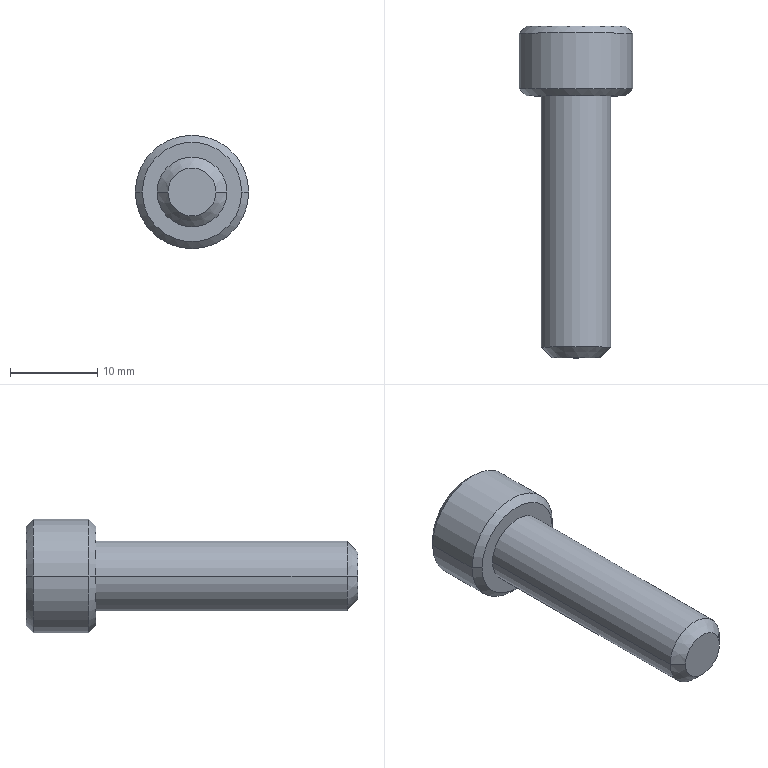Part | STEP file | BB62-M8-30L-1 | 1 solid | 27 faces | box 13 x 38 x 13 mm | volume 2381 mm3 | plane 15 | cone 8 | cylinder 4 | commonest cylinder face diameters 8 x2 13 x2
STEP:
#1=CARTESIAN_POINT('',(-3.,2.02,0.));
#2=VERTEX_POINT('',#1);
#3=CARTESIAN_POINT('',(0.43,4.,0.));
#4=VERTEX_POINT('',#3);
#5=CARTESIAN_POINT('',(-3.,2.02,0.));
#6=DIRECTION('',(0.866,0.5,0.));
#7=VECTOR('',#6,1000.);
#8=LINE('',#5,#7);
#9=EDGE_CURVE('',#2,#4,#8,.T.);
#10=ORIENTED_EDGE('',*,*,#9,.F.);
#11=CARTESIAN_POINT('',(-6.43,4.,0.));
#12=VERTEX_POINT('',#11);
#13=CARTESIAN_POINT('',(-3.,2.02,0.));
#14=DIRECTION('',(-0.866,0.5,0.));
#15=VECTOR('',#14,1000.);
#16=LINE('',#13,#15);
#17=EDGE_CURVE('',#2,#12,#16,.T.);
#18=ORIENTED_EDGE('',*,*,#17,.T.);
#19=CARTESIAN_POINT('',(-5.97,4.,1.715));
#20=VERTEX_POINT('',#19);
#21=CARTESIAN_POINT('',(-3.,4.,0.));
#22=DIRECTION('',(0.,-1.,0.));
#23=DIRECTION('',(-1.,0.,0.));
#24=AXIS2_PLACEMENT_3D('',#21,#22,#23);
#25=CIRCLE('',#24,3.43);
#26=EDGE_CURVE('',#20,#12,#25,.T.);
#27=ORIENTED_EDGE('',*,*,#26,.F.);
#28=CARTESIAN_POINT('',(-3.,4.,3.43));
#29=VERTEX_POINT('',#28);
#30=CARTESIAN_POINT('',(-3.,4.,0.));
#31=DIRECTION('',(0.,-1.,0.));
#32=DIRECTION('',(-1.,0.,0.));
#33=AXIS2_PLACEMENT_3D('',#30,#31,#32);
#34=CIRCLE('',#33,3.43);
#35=EDGE_CURVE('',#29,#20,#34,.T.);
#36=ORIENTED_EDGE('',*,*,#35,.F.);
#37=CARTESIAN_POINT('',(-0.02953,4.,1.715));
#38=VERTEX_POINT('',#37);
#39=CARTESIAN_POINT('',(-3.,4.,0.));
#40=DIRECTION('',(0.,-1.,0.));
#41=DIRECTION('',(-1.,0.,0.));
#42=AXIS2_PLACEMENT_3D('',#39,#40,#41);
#43=CIRCLE('',#42,3.43);
#44=EDGE_CURVE('',#38,#29,#43,.T.);
#45=ORIENTED_EDGE('',*,*,#44,.F.);
#46=CARTESIAN_POINT('',(-3.,4.,0.));
#47=DIRECTION('',(0.,-1.,0.));
#48=DIRECTION('',(-1.,0.,0.));
#49=AXIS2_PLACEMENT_3D('',#46,#47,#48);
#50=CIRCLE('',#49,3.43);
#51=EDGE_CURVE('',#4,#38,#50,.T.);
#52=ORIENTED_EDGE('',*,*,#51,.F.);
#53=EDGE_LOOP('',(#10,#18,#27,#36,#45,#52));
#54=FACE_OUTER_BOUND('',#53,.T.);
#55=CARTESIAN_POINT('',(-3.,1002.02,0.));
#56=DIRECTION('',(0.,1.,0.));
#57=DIRECTION('',(1.,0.,0.));
#58=AXIS2_PLACEMENT_3D('',#55,#56,#57);
#59=CONICAL_SURFACE('',#58,1732.051,1.047);
#60=ADVANCED_FACE('',(#54),#59,.F.);
#61=CARTESIAN_POINT('',(-0.25,-30.,0.));
#62=VERTEX_POINT('',#61);
#63=CARTESIAN_POINT('',(-5.75,-30.,0.));
#64=VERTEX_POINT('',#63);
#65=CARTESIAN_POINT('',(-3.,-30.,0.));
#66=DIRECTION('',(0.,1.,0.));
#67=DIRECTION('',(1.,0.,0.));
#68=AXIS2_PLACEMENT_3D('',#65,#66,#67);
#69=CIRCLE('',#68,2.75);
#70=EDGE_CURVE('',#62,#64,#69,.T.);
#71=ORIENTED_EDGE('',*,*,#70,.T.);
#72=CARTESIAN_POINT('',(-7.,-28.75,0.));
#73=VERTEX_POINT('',#72);
#74=CARTESIAN_POINT('',(-5.75,-30.,0.));
#75=DIRECTION('',(-0.7071,0.7071,0.));
#76=VECTOR('',#75,1000.);
#77=LINE('',#74,#76);
#78=EDGE_CURVE('',#64,#73,#77,.T.);
#79=ORIENTED_EDGE('',*,*,#78,.T.);
#80=CARTESIAN_POINT('',(1.,-28.75,0.));
#81=VERTEX_POINT('',#80);
#82=CARTESIAN_POINT('',(-3.,-28.75,0.));
#83=DIRECTION('',(0.,-1.,0.));
#84=DIRECTION('',(-1.,0.,0.));
#85=AXIS2_PLACEMENT_3D('',#82,#83,#84);
#86=CIRCLE('',#85,4.);
#87=EDGE_CURVE('',#73,#81,#86,.T.);
#88=ORIENTED_EDGE('',*,*,#87,.T.);
#89=CARTESIAN_POINT('',(-0.25,-30.,0.));
#90=DIRECTION('',(0.7071,0.7071,0.));
#91=VECTOR('',#90,1000.);
#92=LINE('',#89,#91);
#93=EDGE_CURVE('',#62,#81,#92,.T.);
#94=ORIENTED_EDGE('',*,*,#93,.F.);
#95=EDGE_LOOP('',(#71,#79,#88,#94));
#96=FACE_OUTER_BOUND('',#95,.T.);
#97=CARTESIAN_POINT('',(-3.,-30.,0.));
#98=DIRECTION('',(0.,1.,0.));
#99=DIRECTION('',(1.,0.,0.));
#100=AXIS2_PLACEMENT_3D('',#97,#98,#99);
#101=CONICAL_SURFACE('',#100,2.75,0.7854);
#102=ADVANCED_FACE('',(#96),#101,.T.);
#103=ORIENTED_EDGE('',*,*,#87,.F.);
#104=CARTESIAN_POINT('',(-7.,0.,0.));
#105=VERTEX_POINT('',#104);
#106=CARTESIAN_POINT('',(-7.,-28.75,0.));
#107=DIRECTION('',(0.,1.,0.));
#108=VECTOR('',#107,1000.);
#109=LINE('',#106,#108);
#110=EDGE_CURVE('',#73,#105,#109,.T.);
#111=ORIENTED_EDGE('',*,*,#110,.T.);
#112=CARTESIAN_POINT('',(1.,0.,0.));
#113=VERTEX_POINT('',#112);
#114=CARTESIAN_POINT('',(-3.,0.,0.));
#115=DIRECTION('',(0.,-1.,0.));
#116=DIRECTION('',(-1.,0.,0.));
#117=AXIS2_PLACEMENT_3D('',#114,#115,#116);
#118=CIRCLE('',#117,4.);
#119=EDGE_CURVE('',#105,#113,#118,.T.);
#120=ORIENTED_EDGE('',*,*,#119,.T.);
#121=CARTESIAN_POINT('',(1.,-28.75,0.));
#122=DIRECTION('',(0.,1.,0.));
#123=VECTOR('',#122,1000.);
#124=LINE('',#121,#123);
#125=EDGE_CURVE('',#81,#113,#124,.T.);
#126=ORIENTED_EDGE('',*,*,#125,.F.);
#127=EDGE_LOOP('',(#103,#111,#120,#126));
#128=FACE_OUTER_BOUND('',#127,.T.);
#129=CARTESIAN_POINT('',(-3.,-28.75,0.));
#130=DIRECTION('',(0.,1.,0.));
#131=DIRECTION('',(1.,0.,0.));
#132=AXIS2_PLACEMENT_3D('',#129,#130,#131);
#133=CYLINDRICAL_SURFACE('',#132,4.);
#134=ADVANCED_FACE('',(#128),#133,.T.);
#135=CARTESIAN_POINT('',(-8.7,8.,0.));
#136=VERTEX_POINT('',#135);
#137=CARTESIAN_POINT('',(2.7,8.,0.));
#138=VERTEX_POINT('',#137);
#139=CARTESIAN_POINT('',(-3.,8.,0.));
#140=DIRECTION('',(0.,-1.,0.));
#141=DIRECTION('',(-1.,0.,0.));
#142=AXIS2_PLACEMENT_3D('',#139,#140,#141);
#143=CIRCLE('',#142,5.7);
#144=EDGE_CURVE('',#136,#138,#143,.T.);
#145=ORIENTED_EDGE('',*,*,#144,.T.);
#146=CARTESIAN_POINT('',(3.5,7.2,0.));
#147=VERTEX_POINT('',#146);
#148=CARTESIAN_POINT('',(3.5,7.2,0.));
#149=DIRECTION('',(0.7071,-0.7071,0.));
#150=VECTOR('',#149,1000.);
#151=LINE('',#148,#150);
#152=EDGE_CURVE('',#138,#147,#151,.T.);
#153=ORIENTED_EDGE('',*,*,#152,.T.);
#154=CARTESIAN_POINT('',(-9.5,7.2,0.));
#155=VERTEX_POINT('',#154);
#156=CARTESIAN_POINT('',(-3.,7.2,0.));
#157=DIRECTION('',(0.,-1.,0.));
#158=DIRECTION('',(-1.,0.,0.));
#159=AXIS2_PLACEMENT_3D('',#156,#157,#158);
#160=CIRCLE('',#159,6.5);
#161=EDGE_CURVE('',#155,#147,#160,.T.);
#162=ORIENTED_EDGE('',*,*,#161,.F.);
#163=CARTESIAN_POINT('',(-9.5,7.2,0.));
#164=DIRECTION('',(-0.7071,-0.7071,0.));
#165=VECTOR('',#164,1000.);
#166=LINE('',#163,#165);
#167=EDGE_CURVE('',#136,#155,#166,.T.);
#168=ORIENTED_EDGE('',*,*,#167,.F.);
#169=EDGE_LOOP('',(#145,#153,#162,#168));
#170=FACE_OUTER_BOUND('',#169,.T.);
#171=CARTESIAN_POINT('',(-3.,7.2,0.));
#172=DIRECTION('',(0.,-1.,0.));
#173=DIRECTION('',(-1.,0.,0.));
#174=AXIS2_PLACEMENT_3D('',#171,#172,#173);
#175=CONICAL_SURFACE('',#174,6.5,0.7854);
#176=ADVANCED_FACE('',(#170),#175,.T.);
#177=ORIENTED_EDGE('',*,*,#161,.T.);
#178=CARTESIAN_POINT('',(3.5,0.8,0.));
#179=VERTEX_POINT('',#178);
#180=CARTESIAN_POINT('',(3.5,1.62,0.));
#181=DIRECTION('',(0.,-1.,0.));
#182=VECTOR('',#181,1000.);
#183=LINE('',#180,#182);
#184=EDGE_CURVE('',#147,#179,#183,.T.);
#185=ORIENTED_EDGE('',*,*,#184,.T.);
#186=CARTESIAN_POINT('',(-9.5,0.8,0.));
#187=VERTEX_POINT('',#186);
#188=CARTESIAN_POINT('',(-3.,0.8,0.));
#189=DIRECTION('',(0.,-1.,0.));
#190=DIRECTION('',(-1.,0.,0.));
#191=AXIS2_PLACEMENT_3D('',#188,#189,#190);
#192=CIRCLE('',#191,6.5);
#193=EDGE_CURVE('',#187,#179,#192,.T.);
#194=ORIENTED_EDGE('',*,*,#193,.F.);
#195=CARTESIAN_POINT('',(-9.5,1.62,0.));
#196=DIRECTION('',(0.,-1.,0.));
#197=VECTOR('',#196,1000.);
#198=LINE('',#195,#197);
#199=EDGE_CURVE('',#155,#187,#198,.T.);
#200=ORIENTED_EDGE('',*,*,#199,.F.);
#201=EDGE_LOOP('',(#177,#185,#194,#200));
#202=FACE_OUTER_BOUND('',#201,.T.);
#203=CARTESIAN_POINT('',(-3.,1.62,0.));
#204=DIRECTION('',(0.,-1.,0.));
#205=DIRECTION('',(-1.,0.,0.));
#206=AXIS2_PLACEMENT_3D('',#203,#204,#205);
#207=CYLINDRICAL_SURFACE('',#206,6.5);
#208=ADVANCED_FACE('',(#202),#207,.T.);
#209=CARTESIAN_POINT('',(-8.7,0.,0.));
#210=VERTEX_POINT('',#209);
#211=CARTESIAN_POINT('',(2.7,0.,0.));
#212=VERTEX_POINT('',#211);
#213=CARTESIAN_POINT('',(-3.,0.,0.));
#214=DIRECTION('',(0.,-1.,0.));
#215=DIRECTION('',(-1.,0.,0.));
#216=AXIS2_PLACEMENT_3D('',#213,#214,#215);
#217=CIRCLE('',#216,5.7);
#218=EDGE_CURVE('',#210,#212,#217,.T.);
#219=ORIENTED_EDGE('',*,*,#218,.F.);
#220=CARTESIAN_POINT('',(-8.7,0.,0.));
#221=DIRECTION('',(-0.7071,0.7071,0.));
#222=VECTOR('',#221,1000.);
#223=LINE('',#220,#222);
#224=EDGE_CURVE('',#210,#187,#223,.T.);
#225=ORIENTED_EDGE('',*,*,#224,.T.);
#226=ORIENTED_EDGE('',*,*,#193,.T.);
#227=CARTESIAN_POINT('',(2.7,0.,0.));
#228=DIRECTION('',(0.7071,0.7071,0.));
#229=VECTOR('',#228,1000.);
#230=LINE('',#227,#229);
#231=EDGE_CURVE('',#212,#179,#230,.T.);
#232=ORIENTED_EDGE('',*,*,#231,.F.);
#233=EDGE_LOOP('',(#219,#225,#226,#232));
#234=FACE_OUTER_BOUND('',#233,.T.);
#235=CARTESIAN_POINT('',(-3.,0.,0.));
#236=DIRECTION('',(0.,1.,0.));
#237=DIRECTION('',(1.,0.,0.));
#238=AXIS2_PLACEMENT_3D('',#235,#236,#237);
#239=CONICAL_SURFACE('',#238,5.7,0.7854);
#240=ADVANCED_FACE('',(#234),#239,.T.);
#241=ORIENTED_EDGE('',*,*,#144,.F.);
#242=CARTESIAN_POINT('',(-3.,8.,0.));
#243=DIRECTION('',(0.,-1.,0.));
#244=DIRECTION('',(-1.,0.,0.));
#245=AXIS2_PLACEMENT_3D('',#242,#243,#244);
#246=CIRCLE('',#245,5.7);
#247=EDGE_CURVE('',#138,#136,#246,.T.);
#248=ORIENTED_EDGE('',*,*,#247,.F.);
#249=EDGE_LOOP('',(#241,#248));
#250=FACE_OUTER_BOUND('',#249,.T.);
#251=CARTESIAN_POINT('',(-3.,8.,-3.43));
#252=VERTEX_POINT('',#251);
#253=CARTESIAN_POINT('',(-5.97,8.,-1.715));
#254=VERTEX_POINT('',#253);
#255=CARTESIAN_POINT('',(-3.,8.,-3.43));
#256=DIRECTION('',(-0.866,0.,0.5));
#257=VECTOR('',#256,1000.);
#258=LINE('',#255,#257);
#259=EDGE_CURVE('',#252,#254,#258,.T.);
#260=ORIENTED_EDGE('',*,*,#259,.F.);
#261=CARTESIAN_POINT('',(-0.02953,8.,-1.715));
#262=VERTEX_POINT('',#261);
#263=CARTESIAN_POINT('',(-0.02953,8.,-1.715));
#264=DIRECTION('',(-0.866,0.,-0.5));
#265=VECTOR('',#264,1000.);
#266=LINE('',#263,#265);
#267=EDGE_CURVE('',#262,#252,#266,.T.);
#268=ORIENTED_EDGE('',*,*,#267,.F.);
#269=CARTESIAN_POINT('',(-0.02953,8.,1.715));
#270=VERTEX_POINT('',#269);
#271=CARTESIAN_POINT('',(-0.02953,8.,1.715));
#272=DIRECTION('',(0.,0.,-1.));
#273=VECTOR('',#272,1000.);
#274=LINE('',#271,#273);
#275=EDGE_CURVE('',#270,#262,#274,.T.);
#276=ORIENTED_EDGE('',*,*,#275,.F.);
#277=CARTESIAN_POINT('',(-3.,8.,3.43));
#278=VERTEX_POINT('',#277);
#279=CARTESIAN_POINT('',(-3.,8.,3.43));
#280=DIRECTION('',(0.866,0.,-0.5));
#281=VECTOR('',#280,1000.);
#282=LINE('',#279,#281);
#283=EDGE_CURVE('',#278,#270,#282,.T.);
#284=ORIENTED_EDGE('',*,*,#283,.F.);
#285=CARTESIAN_POINT('',(-5.97,8.,1.715));
#286=VERTEX_POINT('',#285);
#287=CARTESIAN_POINT('',(-5.97,8.,1.715));
#288=DIRECTION('',(0.866,0.,0.5));
#289=VECTOR('',#288,1000.);
#290=LINE('',#287,#289);
#291=EDGE_CURVE('',#286,#278,#290,.T.);
#292=ORIENTED_EDGE('',*,*,#291,.F.);
#293=CARTESIAN_POINT('',(-5.97,8.,-1.715));
#294=DIRECTION('',(0.,0.,1.));
#295=VECTOR('',#294,1000.);
#296=LINE('',#293,#295);
#297=EDGE_CURVE('',#254,#286,#296,.T.);
#298=ORIENTED_EDGE('',*,*,#297,.F.);
#299=EDGE_LOOP('',(#260,#268,#276,#284,#292,#298));
#300=FACE_BOUND('',#299,.T.);
#301=CARTESIAN_POINT('',(2.7,8.,0.));
#302=DIRECTION('',(0.,1.,0.));
#303=DIRECTION('',(1.,0.,0.));
#304=AXIS2_PLACEMENT_3D('',#301,#302,#303);
#305=PLANE('',#304);
#306=ADVANCED_FACE('',(#250,#300),#305,.T.);
#307=CARTESIAN_POINT('',(-3.,0.,0.));
#308=DIRECTION('',(0.,-1.,0.));
#309=DIRECTION('',(-1.,0.,0.));
#310=AXIS2_PLACEMENT_3D('',#307,#308,#309);
#311=CIRCLE('',#310,4.);
#312=EDGE_CURVE('',#113,#105,#311,.T.);
#313=ORIENTED_EDGE('',*,*,#312,.F.);
#314=ORIENTED_EDGE('',*,*,#119,.F.);
#315=EDGE_LOOP('',(#313,#314));
#316=FACE_BOUND('',#315,.T.);
#317=CARTESIAN_POINT('',(-3.,0.,0.));
#318=DIRECTION('',(0.,-1.,0.));
#319=DIRECTION('',(-1.,0.,0.));
#320=AXIS2_PLACEMENT_3D('',#317,#318,#319);
#321=CIRCLE('',#320,5.7);
#322=EDGE_CURVE('',#212,#210,#321,.T.);
#323=ORIENTED_EDGE('',*,*,#322,.T.);
#324=ORIENTED_EDGE('',*,*,#218,.T.);
#325=EDGE_LOOP('',(#323,#324));
#326=FACE_OUTER_BOUND('',#325,.T.);
#327=CARTESIAN_POINT('',(-3.,0.,0.));
#328=DIRECTION('',(0.,-1.,0.));
#329=DIRECTION('',(-1.,0.,0.));
#330=AXIS2_PLACEMENT_3D('',#327,#328,#329);
#331=PLANE('',#330);
#332=ADVANCED_FACE('',(#316,#326),#331,.T.);
#333=ORIENTED_EDGE('',*,*,#224,.F.);
#334=ORIENTED_EDGE('',*,*,#322,.F.);
#335=ORIENTED_EDGE('',*,*,#231,.T.);
#336=CARTESIAN_POINT('',(-3.,0.8,0.));
#337=DIRECTION('',(0.,-1.,0.));
#338=DIRECTION('',(-1.,0.,0.));
#339=AXIS2_PLACEMENT_3D('',#336,#337,#338);
#340=CIRCLE('',#339,6.5);
#341=EDGE_CURVE('',#179,#187,#340,.T.);
#342=ORIENTED_EDGE('',*,*,#341,.T.);
#343=EDGE_LOOP('',(#333,#334,#335,#342));
#344=FACE_OUTER_BOUND('',#343,.T.);
#345=CARTESIAN_POINT('',(-3.,0.,0.));
#346=DIRECTION('',(0.,1.,0.));
#347=DIRECTION('',(1.,0.,0.));
#348=AXIS2_PLACEMENT_3D('',#345,#346,#347);
#349=CONICAL_SURFACE('',#348,5.7,0.7854);
#350=ADVANCED_FACE('',(#344),#349,.T.);
#351=ORIENTED_EDGE('',*,*,#184,.F.);
#352=CARTESIAN_POINT('',(-3.,7.2,0.));
#353=DIRECTION('',(0.,-1.,0.));
#354=DIRECTION('',(-1.,0.,0.));
#355=AXIS2_PLACEMENT_3D('',#352,#353,#354);
#356=CIRCLE('',#355,6.5);
#357=EDGE_CURVE('',#147,#155,#356,.T.);
#358=ORIENTED_EDGE('',*,*,#357,.T.);
#359=ORIENTED_EDGE('',*,*,#199,.T.);
#360=ORIENTED_EDGE('',*,*,#341,.F.);
#361=EDGE_LOOP('',(#351,#358,#359,#360));
#362=FACE_OUTER_BOUND('',#361,.T.);
#363=CARTESIAN_POINT('',(-3.,1.62,0.));
#364=DIRECTION('',(0.,-1.,0.));
#365=DIRECTION('',(-1.,0.,0.));
#366=AXIS2_PLACEMENT_3D('',#363,#364,#365);
#367=CYLINDRICAL_SURFACE('',#366,6.5);
#368=ADVANCED_FACE('',(#362),#367,.T.);
#369=ORIENTED_EDGE('',*,*,#152,.F.);
#370=ORIENTED_EDGE('',*,*,#247,.T.);
#371=ORIENTED_EDGE('',*,*,#167,.T.);
#372=ORIENTED_EDGE('',*,*,#357,.F.);
#373=EDGE_LOOP('',(#369,#370,#371,#372));
#374=FACE_OUTER_BOUND('',#373,.T.);
#375=CARTESIAN_POINT('',(-3.,7.2,0.));
#376=DIRECTION('',(0.,-1.,0.));
#377=DIRECTION('',(-1.,0.,0.));
#378=AXIS2_PLACEMENT_3D('',#375,#376,#377);
#379=CONICAL_SURFACE('',#378,6.5,0.7854);
#380=ADVANCED_FACE('',(#374),#379,.T.);
#381=ORIENTED_EDGE('',*,*,#110,.F.);
#382=CARTESIAN_POINT('',(-3.,-28.75,0.));
#383=DIRECTION('',(0.,-1.,0.));
#384=DIRECTION('',(-1.,0.,0.));
#385=AXIS2_PLACEMENT_3D('',#382,#383,#384);
#386=CIRCLE('',#385,4.);
#387=EDGE_CURVE('',#81,#73,#386,.T.);
#388=ORIENTED_EDGE('',*,*,#387,.F.);
#389=ORIENTED_EDGE('',*,*,#125,.T.);
#390=ORIENTED_EDGE('',*,*,#312,.T.);
#391=EDGE_LOOP('',(#381,#388,#389,#390));
#392=FACE_OUTER_BOUND('',#391,.T.);
#393=CARTESIAN_POINT('',(-3.,-28.75,0.));
#394=DIRECTION('',(0.,1.,0.));
#395=DIRECTION('',(1.,0.,0.));
#396=AXIS2_PLACEMENT_3D('',#393,#394,#395);
#397=CYLINDRICAL_SURFACE('',#396,4.);
#398=ADVANCED_FACE('',(#392),#397,.T.);
#399=ORIENTED_EDGE('',*,*,#70,.F.);
#400=CARTESIAN_POINT('',(-3.,-30.,0.));
#401=DIRECTION('',(0.,1.,0.));
#402=DIRECTION('',(1.,0.,0.));
#403=AXIS2_PLACEMENT_3D('',#400,#401,#402);
#404=CIRCLE('',#403,2.75);
#405=EDGE_CURVE('',#64,#62,#404,.T.);
#406=ORIENTED_EDGE('',*,*,#405,.F.);
#407=EDGE_LOOP('',(#399,#406));
#408=FACE_OUTER_BOUND('',#407,.T.);
#409=CARTESIAN_POINT('',(-3.,-30.,0.));
#410=DIRECTION('',(0.,-1.,0.));
#411=DIRECTION('',(-1.,0.,0.));
#412=AXIS2_PLACEMENT_3D('',#409,#410,#411);
#413=PLANE('',#412);
#414=ADVANCED_FACE('',(#408),#413,.T.);
#415=ORIENTED_EDGE('',*,*,#78,.F.);
#416=ORIENTED_EDGE('',*,*,#405,.T.);
#417=ORIENTED_EDGE('',*,*,#93,.T.);
#418=ORIENTED_EDGE('',*,*,#387,.T.);
#419=EDGE_LOOP('',(#415,#416,#417,#418));
#420=FACE_OUTER_BOUND('',#419,.T.);
#421=CARTESIAN_POINT('',(-3.,-30.,0.));
#422=DIRECTION('',(0.,1.,0.));
#423=DIRECTION('',(1.,0.,0.));
#424=AXIS2_PLACEMENT_3D('',#421,#422,#423);
#425=CONICAL_SURFACE('',#424,2.75,0.7854);
#426=ADVANCED_FACE('',(#420),#425,.T.);
#427=CARTESIAN_POINT('',(-0.02953,4.,-1.715));
#428=VERTEX_POINT('',#427);
#429=CARTESIAN_POINT('',(-3.,4.,-3.43));
#430=VERTEX_POINT('',#429);
#431=CARTESIAN_POINT('',(-0.02953,4.,-1.715));
#432=DIRECTION('',(-0.866,0.,-0.5));
#433=VECTOR('',#432,1000.);
#434=LINE('',#431,#433);
#435=EDGE_CURVE('',#428,#430,#434,.T.);
#436=ORIENTED_EDGE('',*,*,#435,.F.);
#437=CARTESIAN_POINT('',(-0.02953,8.,-1.715));
#438=DIRECTION('',(0.,-1.,0.));
#439=VECTOR('',#438,1000.);
#440=LINE('',#437,#439);
#441=EDGE_CURVE('',#262,#428,#440,.T.);
#442=ORIENTED_EDGE('',*,*,#441,.F.);
#443=ORIENTED_EDGE('',*,*,#267,.T.);
#444=CARTESIAN_POINT('',(-3.,8.,-3.43));
#445=DIRECTION('',(0.,-1.,0.));
#446=VECTOR('',#445,1000.);
#447=LINE('',#444,#446);
#448=EDGE_CURVE('',#252,#430,#447,.T.);
#449=ORIENTED_EDGE('',*,*,#448,.T.);
#450=EDGE_LOOP('',(#436,#442,#443,#449));
#451=FACE_OUTER_BOUND('',#450,.T.);
#452=CARTESIAN_POINT('',(-0.02953,8.,-1.715));
#453=DIRECTION('',(-0.5,0.,0.866));
#454=DIRECTION('',(0.866,0.,0.5));
#455=AXIS2_PLACEMENT_3D('',#452,#453,#454);
#456=PLANE('',#455);
#457=ADVANCED_FACE('',(#451),#456,.T.);
#458=CARTESIAN_POINT('',(-5.97,4.,-1.715));
#459=VERTEX_POINT('',#458);
#460=CARTESIAN_POINT('',(-3.,4.,-3.43));
#461=DIRECTION('',(-0.866,0.,0.5));
#462=VECTOR('',#461,1000.);
#463=LINE('',#460,#462);
#464=EDGE_CURVE('',#430,#459,#463,.T.);
#465=ORIENTED_EDGE('',*,*,#464,.F.);
#466=ORIENTED_EDGE('',*,*,#448,.F.);
#467=ORIENTED_EDGE('',*,*,#259,.T.);
#468=CARTESIAN_POINT('',(-5.97,8.,-1.715));
#469=DIRECTION('',(0.,-1.,0.));
#470=VECTOR('',#469,1000.);
#471=LINE('',#468,#470);
#472=EDGE_CURVE('',#254,#459,#471,.T.);
#473=ORIENTED_EDGE('',*,*,#472,.T.);
#474=EDGE_LOOP('',(#465,#466,#467,#473));
#475=FACE_OUTER_BOUND('',#474,.T.);
#476=CARTESIAN_POINT('',(-3.,8.,-3.43));
#477=DIRECTION('',(0.5,0.,0.866));
#478=DIRECTION('',(0.866,0.,-0.5));
#479=AXIS2_PLACEMENT_3D('',#476,#477,#478);
#480=PLANE('',#479);
#481=ADVANCED_FACE('',(#475),#480,.T.);
#482=CARTESIAN_POINT('',(-5.97,4.,-1.715));
#483=DIRECTION('',(0.,0.,1.));
#484=VECTOR('',#483,1000.);
#485=LINE('',#482,#484);
#486=EDGE_CURVE('',#459,#20,#485,.T.);
#487=ORIENTED_EDGE('',*,*,#486,.F.);
#488=ORIENTED_EDGE('',*,*,#472,.F.);
#489=ORIENTED_EDGE('',*,*,#297,.T.);
#490=CARTESIAN_POINT('',(-5.97,8.,1.715));
#491=DIRECTION('',(0.,-1.,0.));
#492=VECTOR('',#491,1000.);
#493=LINE('',#490,#492);
#494=EDGE_CURVE('',#286,#20,#493,.T.);
#495=ORIENTED_EDGE('',*,*,#494,.T.);
#496=EDGE_LOOP('',(#487,#488,#489,#495));
#497=FACE_OUTER_BOUND('',#496,.T.);
#498=CARTESIAN_POINT('',(-5.97,8.,-1.715));
#499=DIRECTION('',(1.,0.,0.));
#500=DIRECTION('',(0.,0.,-1.));
#501=AXIS2_PLACEMENT_3D('',#498,#499,#500);
#502=PLANE('',#501);
#503=ADVANCED_FACE('',(#497),#502,.T.);
#504=CARTESIAN_POINT('',(-5.97,4.,1.715));
#505=DIRECTION('',(0.866,0.,0.5));
#506=VECTOR('',#505,1000.);
#507=LINE('',#504,#506);
#508=EDGE_CURVE('',#20,#29,#507,.T.);
#509=ORIENTED_EDGE('',*,*,#508,.F.);
#510=ORIENTED_EDGE('',*,*,#494,.F.);
#511=ORIENTED_EDGE('',*,*,#291,.T.);
#512=CARTESIAN_POINT('',(-3.,8.,3.43));
#513=DIRECTION('',(0.,-1.,0.));
#514=VECTOR('',#513,1000.);
#515=LINE('',#512,#514);
#516=EDGE_CURVE('',#278,#29,#515,.T.);
#517=ORIENTED_EDGE('',*,*,#516,.T.);
#518=EDGE_LOOP('',(#509,#510,#511,#517));
#519=FACE_OUTER_BOUND('',#518,.T.);
#520=CARTESIAN_POINT('',(-5.97,8.,1.715));
#521=DIRECTION('',(0.5,0.,-0.866));
#522=DIRECTION('',(-0.866,0.,-0.5));
#523=AXIS2_PLACEMENT_3D('',#520,#521,#522);
#524=PLANE('',#523);
#525=ADVANCED_FACE('',(#519),#524,.T.);
#526=CARTESIAN_POINT('',(-3.,4.,3.43));
#527=DIRECTION('',(0.866,0.,-0.5));
#528=VECTOR('',#527,1000.);
#529=LINE('',#526,#528);
#530=EDGE_CURVE('',#29,#38,#529,.T.);
#531=ORIENTED_EDGE('',*,*,#530,.F.);
#532=ORIENTED_EDGE('',*,*,#516,.F.);
#533=ORIENTED_EDGE('',*,*,#283,.T.);
#534=CARTESIAN_POINT('',(-0.02953,8.,1.715));
#535=DIRECTION('',(0.,-1.,0.));
#536=VECTOR('',#535,1000.);
#537=LINE('',#534,#536);
#538=EDGE_CURVE('',#270,#38,#537,.T.);
#539=ORIENTED_EDGE('',*,*,#538,.T.);
#540=EDGE_LOOP('',(#531,#532,#533,#539));
#541=FACE_OUTER_BOUND('',#540,.T.);
#542=CARTESIAN_POINT('',(-3.,8.,3.43));
#543=DIRECTION('',(-0.5,0.,-0.866));
#544=DIRECTION('',(-0.866,0.,0.5));
#545=AXIS2_PLACEMENT_3D('',#542,#543,#544);
#546=PLANE('',#545);
#547=ADVANCED_FACE('',(#541),#546,.T.);
#548=CARTESIAN_POINT('',(-0.02953,4.,1.715));
#549=DIRECTION('',(0.,0.,-1.));
#550=VECTOR('',#549,1000.);
#551=LINE('',#548,#550);
#552=EDGE_CURVE('',#38,#428,#551,.T.);
#553=ORIENTED_EDGE('',*,*,#552,.F.);
#554=ORIENTED_EDGE('',*,*,#538,.F.);
#555=ORIENTED_EDGE('',*,*,#275,.T.);
#556=ORIENTED_EDGE('',*,*,#441,.T.);
#557=EDGE_LOOP('',(#553,#554,#555,#556));
#558=FACE_OUTER_BOUND('',#557,.T.);
#559=CARTESIAN_POINT('',(-0.02953,8.,1.715));
#560=DIRECTION('',(-1.,0.,0.));
#561=DIRECTION('',(0.,0.,1.));
#562=AXIS2_PLACEMENT_3D('',#559,#560,#561);
#563=PLANE('',#562);
#564=ADVANCED_FACE('',(#558),#563,.T.);
#565=ORIENTED_EDGE('',*,*,#435,.T.);
#566=CARTESIAN_POINT('',(-3.,4.,0.));
#567=DIRECTION('',(0.,-1.,0.));
#568=DIRECTION('',(-1.,0.,0.));
#569=AXIS2_PLACEMENT_3D('',#566,#567,#568);
#570=CIRCLE('',#569,3.43);
#571=EDGE_CURVE('',#430,#428,#570,.T.);
#572=ORIENTED_EDGE('',*,*,#571,.T.);
#573=EDGE_LOOP('',(#565,#572));
#574=FACE_OUTER_BOUND('',#573,.T.);
#575=CARTESIAN_POINT('',(-3.,4.,0.));
#576=DIRECTION('',(0.,1.,0.));
#577=DIRECTION('',(1.,0.,0.));
#578=AXIS2_PLACEMENT_3D('',#575,#576,#577);
#579=PLANE('',#578);
#580=ADVANCED_FACE('',(#574),#579,.F.);
#581=ORIENTED_EDGE('',*,*,#552,.T.);
#582=CARTESIAN_POINT('',(-3.,4.,0.));
#583=DIRECTION('',(0.,-1.,0.));
#584=DIRECTION('',(-1.,0.,0.));
#585=AXIS2_PLACEMENT_3D('',#582,#583,#584);
#586=CIRCLE('',#585,3.43);
#587=EDGE_CURVE('',#428,#4,#586,.T.);
#588=ORIENTED_EDGE('',*,*,#587,.T.);
#589=ORIENTED_EDGE('',*,*,#51,.T.);
#590=EDGE_LOOP('',(#581,#588,#589));
#591=FACE_OUTER_BOUND('',#590,.T.);
#592=CARTESIAN_POINT('',(-3.,4.,0.));
#593=DIRECTION('',(0.,1.,0.));
#594=DIRECTION('',(1.,0.,0.));
#595=AXIS2_PLACEMENT_3D('',#592,#593,#594);
#596=PLANE('',#595);
#597=ADVANCED_FACE('',(#591),#596,.F.);
#598=ORIENTED_EDGE('',*,*,#530,.T.);
#599=ORIENTED_EDGE('',*,*,#44,.T.);
#600=EDGE_LOOP('',(#598,#599));
#601=FACE_OUTER_BOUND('',#600,.T.);
#602=CARTESIAN_POINT('',(-3.,4.,0.));
#603=DIRECTION('',(0.,1.,0.));
#604=DIRECTION('',(1.,0.,0.));
#605=AXIS2_PLACEMENT_3D('',#602,#603,#604);
#606=PLANE('',#605);
#607=ADVANCED_FACE('',(#601),#606,.F.);
#608=ORIENTED_EDGE('',*,*,#508,.T.);
#609=ORIENTED_EDGE('',*,*,#35,.T.);
#610=EDGE_LOOP('',(#608,#609));
#611=FACE_OUTER_BOUND('',#610,.T.);
#612=CARTESIAN_POINT('',(-3.,4.,0.));
#613=DIRECTION('',(0.,1.,0.));
#614=DIRECTION('',(1.,0.,0.));
#615=AXIS2_PLACEMENT_3D('',#612,#613,#614);
#616=PLANE('',#615);
#617=ADVANCED_FACE('',(#611),#616,.F.);
#618=ORIENTED_EDGE('',*,*,#486,.T.);
#619=ORIENTED_EDGE('',*,*,#26,.T.);
#620=CARTESIAN_POINT('',(-3.,4.,0.));
#621=DIRECTION('',(0.,-1.,0.));
#622=DIRECTION('',(-1.,0.,0.));
#623=AXIS2_PLACEMENT_3D('',#620,#621,#622);
#624=CIRCLE('',#623,3.43);
#625=EDGE_CURVE('',#12,#459,#624,.T.);
#626=ORIENTED_EDGE('',*,*,#625,.T.);
#627=EDGE_LOOP('',(#618,#619,#626));
#628=FACE_OUTER_BOUND('',#627,.T.);
#629=CARTESIAN_POINT('',(-3.,4.,0.));
#630=DIRECTION('',(0.,1.,0.));
#631=DIRECTION('',(1.,0.,0.));
#632=AXIS2_PLACEMENT_3D('',#629,#630,#631);
#633=PLANE('',#632);
#634=ADVANCED_FACE('',(#628),#633,.F.);
#635=ORIENTED_EDGE('',*,*,#464,.T.);
#636=CARTESIAN_POINT('',(-3.,4.,0.));
#637=DIRECTION('',(0.,-1.,0.));
#638=DIRECTION('',(-1.,0.,0.));
#639=AXIS2_PLACEMENT_3D('',#636,#637,#638);
#640=CIRCLE('',#639,3.43);
#641=EDGE_CURVE('',#459,#430,#640,.T.);
#642=ORIENTED_EDGE('',*,*,#641,.T.);
#643=EDGE_LOOP('',(#635,#642));
#644=FACE_OUTER_BOUND('',#643,.T.);
#645=CARTESIAN_POINT('',(-3.,4.,0.));
#646=DIRECTION('',(0.,1.,0.));
#647=DIRECTION('',(1.,0.,0.));
#648=AXIS2_PLACEMENT_3D('',#645,#646,#647);
#649=PLANE('',#648);
#650=ADVANCED_FACE('',(#644),#649,.F.);
#651=ORIENTED_EDGE('',*,*,#17,.F.);
#652=ORIENTED_EDGE('',*,*,#9,.T.);
#653=ORIENTED_EDGE('',*,*,#587,.F.);
#654=ORIENTED_EDGE('',*,*,#571,.F.);
#655=ORIENTED_EDGE('',*,*,#641,.F.);
#656=ORIENTED_EDGE('',*,*,#625,.F.);
#657=EDGE_LOOP('',(#651,#652,#653,#654,#655,#656));
#658=FACE_OUTER_BOUND('',#657,.T.);
#659=CARTESIAN_POINT('',(-3.,1002.02,0.));
#660=DIRECTION('',(0.,1.,0.));
#661=DIRECTION('',(1.,0.,0.));
#662=AXIS2_PLACEMENT_3D('',#659,#660,#661);
#663=CONICAL_SURFACE('',#662,1732.051,1.047);
#664=ADVANCED_FACE('',(#658),#663,.F.);
#665=CLOSED_SHELL('',(#60,#102,#134,#176,#208,#240,#306,#332,#350,#368,#380,#398,#414,#426,#457,#481,#503,#525,#547,#564,#580,#597,#607,#617,#634,#650,#664));
#666=MANIFOLD_SOLID_BREP('',#665);
#667=CARTESIAN_POINT('',(0.,0.,0.));
#668=DIRECTION('',(0.,0.,1.));
#669=DIRECTION('',(1.,0.,0.));
#670=AXIS2_PLACEMENT_3D('',#667,#668,#669);
#671=(LENGTH_UNIT()NAMED_UNIT(*)SI_UNIT(.MILLI.,.METRE.));
#672=UNCERTAINTY_MEASURE_WITH_UNIT(LENGTH_MEASURE(0.00001),#671,'','');
#673=(NAMED_UNIT(*)PLANE_ANGLE_UNIT()SI_UNIT($,.RADIAN.));
#674=(NAMED_UNIT(*)SI_UNIT($,.STERADIAN.)SOLID_ANGLE_UNIT());
#675=(GEOMETRIC_REPRESENTATION_CONTEXT(3)GLOBAL_UNCERTAINTY_ASSIGNED_CONTEXT((#672))GLOBAL_UNIT_ASSIGNED_CONTEXT((#671,#673,#674))REPRESENTATION_CONTEXT('',''));
#676=ADVANCED_BREP_SHAPE_REPRESENTATION('',(#666,#670),#675);